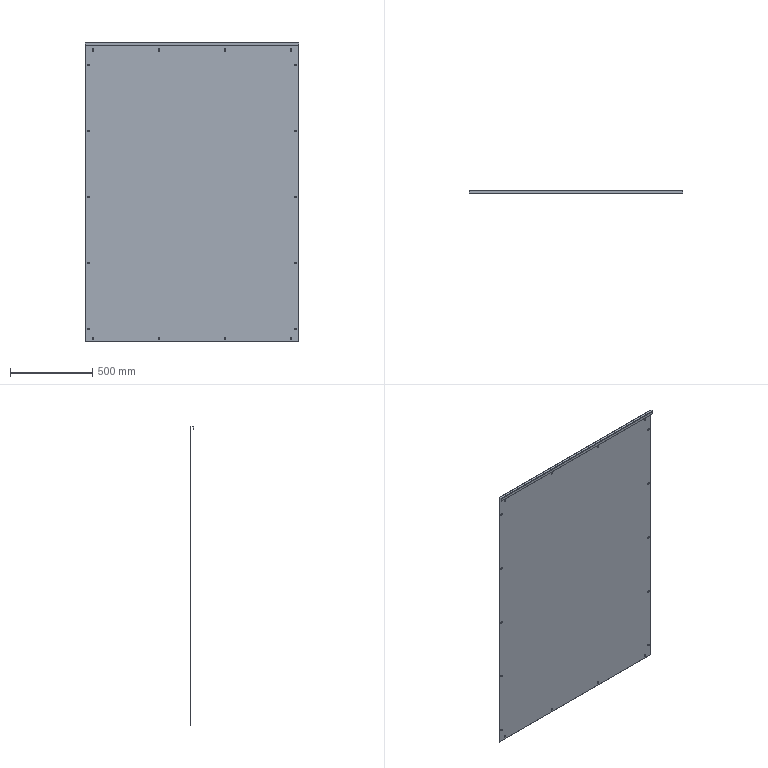Part | NX | features BREP 1 | 1 solid | 102 faces | box 1296 x 20 x 1818 mm | volume 3599358 mm3 | plane 54 | cylinder 48 | commonest cylinder face diameters 7 x46 4 x2